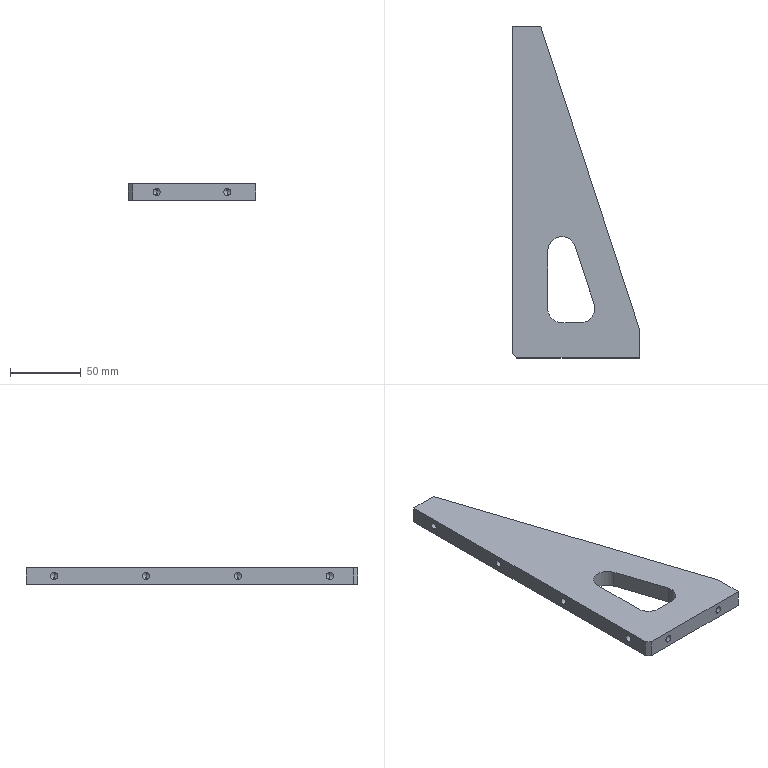Part | STEP file | PN_0020 | 1 solid | 38 faces | box 90 x 235 x 12 mm | volume 142926 mm3 | cylinder 15 | cone 12 | plane 11 | commonest cylinder face diameters 5 x12 20 x3